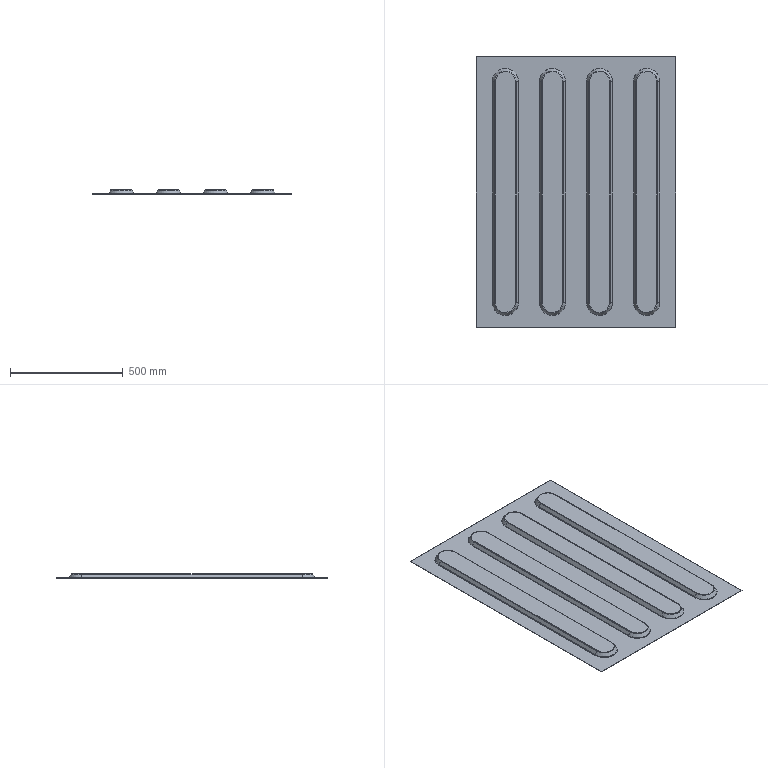Part | STEP file | 750038166 | 1 solid | 111 faces | box 884 x 1200 x 19.9 mm | volume 1728318 mm3 | cylinder 32 | spline 32 | plane 30 | cone 17 | commonest cylinder face diameters 4 x16 7 x16